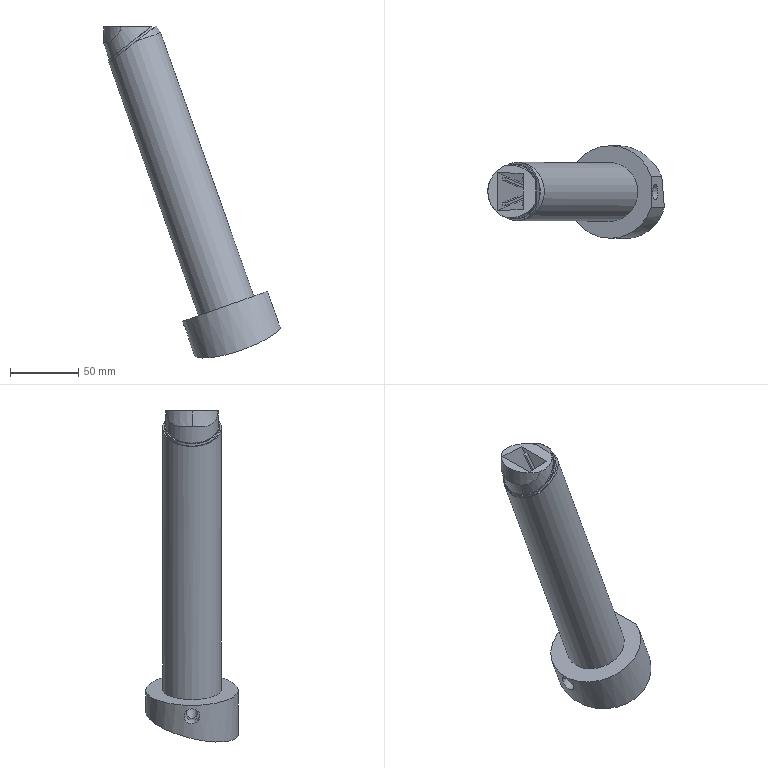Part | STEP file | SLIDE1-INSERT1_id642_x_t | 1 solid | 52 faces | box 129.599 x 68 x 243.479 mm | volume 360421 mm3 | plane 36 | cylinder 9 | cone 5 | other 2 | commonest cylinder face diameters 8 x2 12 x1 12.5 x1 13.5 x1 38.684 x1 40.211 x1